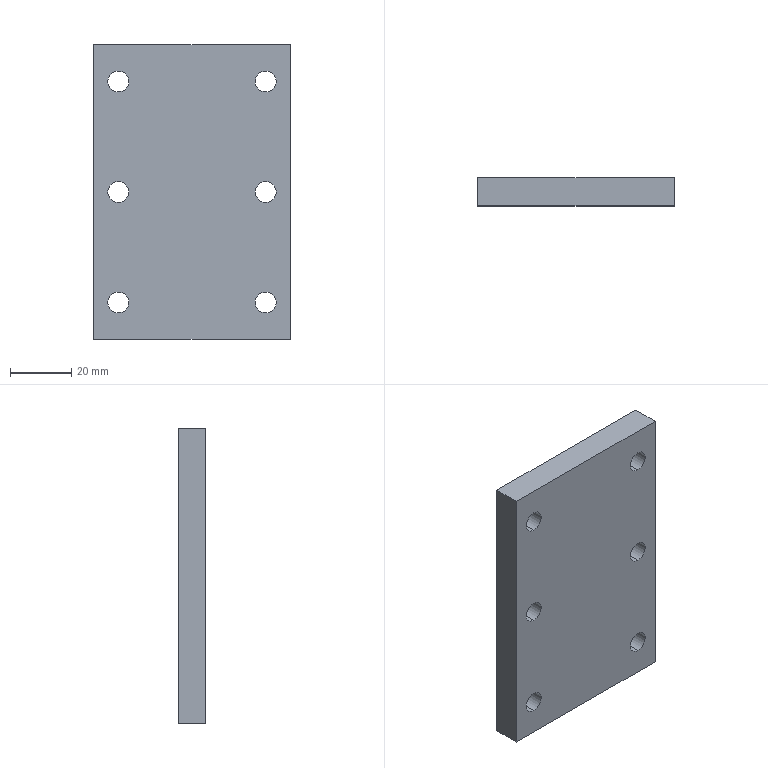Part | STEP file | 0245_215_Plate | 1 solid | 18 faces | box 64 x 9 x 96 mm | volume 53335 mm3 | cylinder 12 | plane 6 | commonest cylinder face diameters 6.8 x12